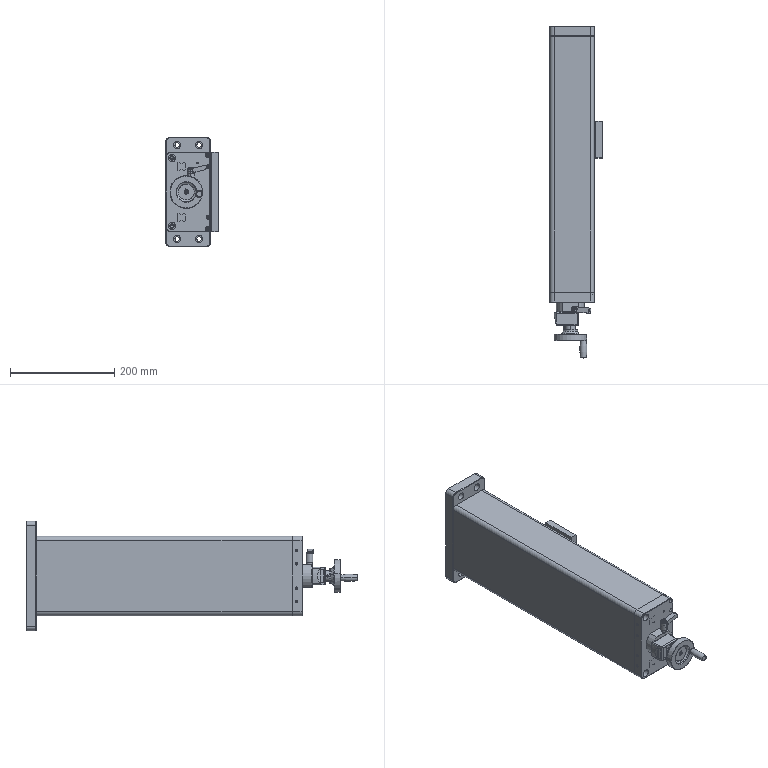Part | SolidWorks | 15 solids | 3606 faces | volume 3066920 mm3 | plane 2728 | cylinder 525 | spline 196 | cone 148 | torus 7 | sphere 2 | commonest cylinder face diameters 4.5 x84 7.5 x72 4 x29 3 x24 8 x21 5 x20